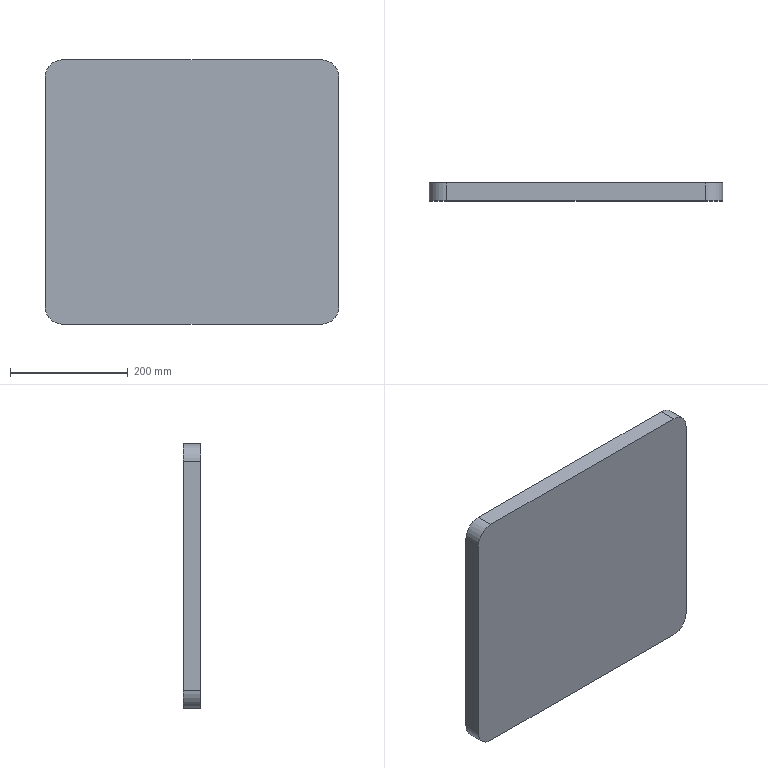Part | SolidWorks | features Extrusion 1, ICE 1 | 1 solid | 19 faces | box 500 x 30 x 450 mm | volume 1262737 mm3 | plane 11 | cylinder 8 | commonest cylinder face diameters 60 x8
STEP:
#1=CARTESIAN_POINT('',(-250.,0.,195.));
#2=VERTEX_POINT('',#1);
#3=CARTESIAN_POINT('',(-220.,0.,225.));
#4=VERTEX_POINT('',#3);
#5=CARTESIAN_POINT('',(-220.,0.,195.));
#6=DIRECTION('',(0.,1.,0.));
#7=DIRECTION('',(0.,0.,-1.));
#8=AXIS2_PLACEMENT_3D('',#5,#6,#7);
#9=CIRCLE('',#8,30.);
#10=EDGE_CURVE('',#2,#4,#9,.T.);
#11=ORIENTED_EDGE('',*,*,#10,.T.);
#12=CARTESIAN_POINT('',(-220.,30.,225.));
#13=VERTEX_POINT('',#12);
#14=CARTESIAN_POINT('',(-220.,30.,225.));
#15=DIRECTION('',(0.,-1.,0.));
#16=VECTOR('',#15,1000.);
#17=LINE('',#14,#16);
#18=EDGE_CURVE('',#13,#4,#17,.T.);
#19=ORIENTED_EDGE('',*,*,#18,.F.);
#20=CARTESIAN_POINT('',(-250.,30.,195.));
#21=VERTEX_POINT('',#20);
#22=CARTESIAN_POINT('',(-220.,30.,195.));
#23=DIRECTION('',(0.,1.,0.));
#24=DIRECTION('',(0.,0.,-1.));
#25=AXIS2_PLACEMENT_3D('',#22,#23,#24);
#26=CIRCLE('',#25,30.);
#27=EDGE_CURVE('',#21,#13,#26,.T.);
#28=ORIENTED_EDGE('',*,*,#27,.F.);
#29=CARTESIAN_POINT('',(-250.,30.,195.));
#30=DIRECTION('',(0.,-1.,0.));
#31=VECTOR('',#30,1000.);
#32=LINE('',#29,#31);
#33=EDGE_CURVE('',#21,#2,#32,.T.);
#34=ORIENTED_EDGE('',*,*,#33,.T.);
#35=EDGE_LOOP('',(#11,#19,#28,#34));
#36=FACE_OUTER_BOUND('',#35,.T.);
#37=CARTESIAN_POINT('',(-220.,30.,195.));
#38=DIRECTION('',(0.,-1.,0.));
#39=DIRECTION('',(0.,0.,-1.));
#40=AXIS2_PLACEMENT_3D('',#37,#38,#39);
#41=CYLINDRICAL_SURFACE('',#40,30.);
#42=ADVANCED_FACE('',(#36),#41,.T.);
#43=CARTESIAN_POINT('',(220.,0.,225.));
#44=VERTEX_POINT('',#43);
#45=CARTESIAN_POINT('',(-220.,0.,225.));
#46=DIRECTION('',(1.,0.,0.));
#47=VECTOR('',#46,1000.);
#48=LINE('',#45,#47);
#49=EDGE_CURVE('',#4,#44,#48,.T.);
#50=ORIENTED_EDGE('',*,*,#49,.T.);
#51=CARTESIAN_POINT('',(220.,30.,225.));
#52=VERTEX_POINT('',#51);
#53=CARTESIAN_POINT('',(220.,30.,225.));
#54=DIRECTION('',(0.,-1.,0.));
#55=VECTOR('',#54,1000.);
#56=LINE('',#53,#55);
#57=EDGE_CURVE('',#52,#44,#56,.T.);
#58=ORIENTED_EDGE('',*,*,#57,.F.);
#59=CARTESIAN_POINT('',(-220.,30.,225.));
#60=DIRECTION('',(1.,0.,0.));
#61=VECTOR('',#60,1000.);
#62=LINE('',#59,#61);
#63=EDGE_CURVE('',#13,#52,#62,.T.);
#64=ORIENTED_EDGE('',*,*,#63,.F.);
#65=ORIENTED_EDGE('',*,*,#18,.T.);
#66=EDGE_LOOP('',(#50,#58,#64,#65));
#67=FACE_OUTER_BOUND('',#66,.T.);
#68=CARTESIAN_POINT('',(-220.,30.,225.));
#69=DIRECTION('',(0.,0.,-1.));
#70=DIRECTION('',(-1.,0.,0.));
#71=AXIS2_PLACEMENT_3D('',#68,#69,#70);
#72=PLANE('',#71);
#73=ADVANCED_FACE('',(#67),#72,.F.);
#74=CARTESIAN_POINT('',(250.,0.,195.));
#75=VERTEX_POINT('',#74);
#76=CARTESIAN_POINT('',(220.,0.,195.));
#77=DIRECTION('',(0.,1.,0.));
#78=DIRECTION('',(0.,0.,-1.));
#79=AXIS2_PLACEMENT_3D('',#76,#77,#78);
#80=CIRCLE('',#79,30.);
#81=EDGE_CURVE('',#44,#75,#80,.T.);
#82=ORIENTED_EDGE('',*,*,#81,.T.);
#83=CARTESIAN_POINT('',(250.,30.,195.));
#84=VERTEX_POINT('',#83);
#85=CARTESIAN_POINT('',(250.,30.,195.));
#86=DIRECTION('',(0.,-1.,0.));
#87=VECTOR('',#86,1000.);
#88=LINE('',#85,#87);
#89=EDGE_CURVE('',#84,#75,#88,.T.);
#90=ORIENTED_EDGE('',*,*,#89,.F.);
#91=CARTESIAN_POINT('',(220.,30.,195.));
#92=DIRECTION('',(0.,1.,0.));
#93=DIRECTION('',(0.,0.,-1.));
#94=AXIS2_PLACEMENT_3D('',#91,#92,#93);
#95=CIRCLE('',#94,30.);
#96=EDGE_CURVE('',#52,#84,#95,.T.);
#97=ORIENTED_EDGE('',*,*,#96,.F.);
#98=ORIENTED_EDGE('',*,*,#57,.T.);
#99=EDGE_LOOP('',(#82,#90,#97,#98));
#100=FACE_OUTER_BOUND('',#99,.T.);
#101=CARTESIAN_POINT('',(220.,30.,195.));
#102=DIRECTION('',(0.,-1.,0.));
#103=DIRECTION('',(0.,0.,-1.));
#104=AXIS2_PLACEMENT_3D('',#101,#102,#103);
#105=CYLINDRICAL_SURFACE('',#104,30.);
#106=ADVANCED_FACE('',(#100),#105,.T.);
#107=CARTESIAN_POINT('',(250.,0.,-195.));
#108=VERTEX_POINT('',#107);
#109=CARTESIAN_POINT('',(250.,0.,-195.));
#110=DIRECTION('',(0.,0.,-1.));
#111=VECTOR('',#110,1000.);
#112=LINE('',#109,#111);
#113=EDGE_CURVE('',#75,#108,#112,.T.);
#114=ORIENTED_EDGE('',*,*,#113,.T.);
#115=CARTESIAN_POINT('',(250.,30.,-195.));
#116=VERTEX_POINT('',#115);
#117=CARTESIAN_POINT('',(250.,30.,-195.));
#118=DIRECTION('',(0.,-1.,0.));
#119=VECTOR('',#118,1000.);
#120=LINE('',#117,#119);
#121=EDGE_CURVE('',#116,#108,#120,.T.);
#122=ORIENTED_EDGE('',*,*,#121,.F.);
#123=CARTESIAN_POINT('',(250.,30.,-195.));
#124=DIRECTION('',(0.,0.,-1.));
#125=VECTOR('',#124,1000.);
#126=LINE('',#123,#125);
#127=EDGE_CURVE('',#84,#116,#126,.T.);
#128=ORIENTED_EDGE('',*,*,#127,.F.);
#129=ORIENTED_EDGE('',*,*,#89,.T.);
#130=EDGE_LOOP('',(#114,#122,#128,#129));
#131=FACE_OUTER_BOUND('',#130,.T.);
#132=CARTESIAN_POINT('',(250.,30.,-195.));
#133=DIRECTION('',(-1.,0.,0.));
#134=DIRECTION('',(0.,0.,1.));
#135=AXIS2_PLACEMENT_3D('',#132,#133,#134);
#136=PLANE('',#135);
#137=ADVANCED_FACE('',(#131),#136,.F.);
#138=CARTESIAN_POINT('',(220.,0.,-225.));
#139=VERTEX_POINT('',#138);
#140=CARTESIAN_POINT('',(220.,0.,-195.));
#141=DIRECTION('',(0.,1.,0.));
#142=DIRECTION('',(0.,0.,1.));
#143=AXIS2_PLACEMENT_3D('',#140,#141,#142);
#144=CIRCLE('',#143,30.);
#145=EDGE_CURVE('',#108,#139,#144,.T.);
#146=ORIENTED_EDGE('',*,*,#145,.T.);
#147=CARTESIAN_POINT('',(220.,30.,-225.));
#148=VERTEX_POINT('',#147);
#149=CARTESIAN_POINT('',(220.,30.,-225.));
#150=DIRECTION('',(0.,-1.,0.));
#151=VECTOR('',#150,1000.);
#152=LINE('',#149,#151);
#153=EDGE_CURVE('',#148,#139,#152,.T.);
#154=ORIENTED_EDGE('',*,*,#153,.F.);
#155=CARTESIAN_POINT('',(220.,30.,-195.));
#156=DIRECTION('',(0.,1.,0.));
#157=DIRECTION('',(0.,0.,1.));
#158=AXIS2_PLACEMENT_3D('',#155,#156,#157);
#159=CIRCLE('',#158,30.);
#160=EDGE_CURVE('',#116,#148,#159,.T.);
#161=ORIENTED_EDGE('',*,*,#160,.F.);
#162=ORIENTED_EDGE('',*,*,#121,.T.);
#163=EDGE_LOOP('',(#146,#154,#161,#162));
#164=FACE_OUTER_BOUND('',#163,.T.);
#165=CARTESIAN_POINT('',(220.,30.,-195.));
#166=DIRECTION('',(0.,-1.,0.));
#167=DIRECTION('',(0.,0.,-1.));
#168=AXIS2_PLACEMENT_3D('',#165,#166,#167);
#169=CYLINDRICAL_SURFACE('',#168,30.);
#170=ADVANCED_FACE('',(#164),#169,.T.);
#171=CARTESIAN_POINT('',(-220.,0.,-225.));
#172=VERTEX_POINT('',#171);
#173=CARTESIAN_POINT('',(-220.,0.,-225.));
#174=DIRECTION('',(-1.,0.,0.));
#175=VECTOR('',#174,1000.);
#176=LINE('',#173,#175);
#177=EDGE_CURVE('',#139,#172,#176,.T.);
#178=ORIENTED_EDGE('',*,*,#177,.T.);
#179=CARTESIAN_POINT('',(-220.,30.,-225.));
#180=VERTEX_POINT('',#179);
#181=CARTESIAN_POINT('',(-220.,30.,-225.));
#182=DIRECTION('',(0.,-1.,0.));
#183=VECTOR('',#182,1000.);
#184=LINE('',#181,#183);
#185=EDGE_CURVE('',#180,#172,#184,.T.);
#186=ORIENTED_EDGE('',*,*,#185,.F.);
#187=CARTESIAN_POINT('',(-220.,30.,-225.));
#188=DIRECTION('',(-1.,0.,0.));
#189=VECTOR('',#188,1000.);
#190=LINE('',#187,#189);
#191=EDGE_CURVE('',#148,#180,#190,.T.);
#192=ORIENTED_EDGE('',*,*,#191,.F.);
#193=ORIENTED_EDGE('',*,*,#153,.T.);
#194=EDGE_LOOP('',(#178,#186,#192,#193));
#195=FACE_OUTER_BOUND('',#194,.T.);
#196=CARTESIAN_POINT('',(-220.,30.,-225.));
#197=DIRECTION('',(0.,0.,1.));
#198=DIRECTION('',(1.,0.,0.));
#199=AXIS2_PLACEMENT_3D('',#196,#197,#198);
#200=PLANE('',#199);
#201=ADVANCED_FACE('',(#195),#200,.F.);
#202=CARTESIAN_POINT('',(-250.,0.,-195.));
#203=VERTEX_POINT('',#202);
#204=CARTESIAN_POINT('',(-220.,0.,-195.));
#205=DIRECTION('',(0.,1.,0.));
#206=DIRECTION('',(0.,0.,1.));
#207=AXIS2_PLACEMENT_3D('',#204,#205,#206);
#208=CIRCLE('',#207,30.);
#209=EDGE_CURVE('',#172,#203,#208,.T.);
#210=ORIENTED_EDGE('',*,*,#209,.T.);
#211=CARTESIAN_POINT('',(-250.,30.,-195.));
#212=VERTEX_POINT('',#211);
#213=CARTESIAN_POINT('',(-250.,30.,-195.));
#214=DIRECTION('',(0.,-1.,0.));
#215=VECTOR('',#214,1000.);
#216=LINE('',#213,#215);
#217=EDGE_CURVE('',#212,#203,#216,.T.);
#218=ORIENTED_EDGE('',*,*,#217,.F.);
#219=CARTESIAN_POINT('',(-220.,30.,-195.));
#220=DIRECTION('',(0.,1.,0.));
#221=DIRECTION('',(0.,0.,1.));
#222=AXIS2_PLACEMENT_3D('',#219,#220,#221);
#223=CIRCLE('',#222,30.);
#224=EDGE_CURVE('',#180,#212,#223,.T.);
#225=ORIENTED_EDGE('',*,*,#224,.F.);
#226=ORIENTED_EDGE('',*,*,#185,.T.);
#227=EDGE_LOOP('',(#210,#218,#225,#226));
#228=FACE_OUTER_BOUND('',#227,.T.);
#229=CARTESIAN_POINT('',(-220.,30.,-195.));
#230=DIRECTION('',(0.,-1.,0.));
#231=DIRECTION('',(0.,0.,-1.));
#232=AXIS2_PLACEMENT_3D('',#229,#230,#231);
#233=CYLINDRICAL_SURFACE('',#232,30.);
#234=ADVANCED_FACE('',(#228),#233,.T.);
#235=CARTESIAN_POINT('',(-250.,0.,-195.));
#236=DIRECTION('',(0.,0.,1.));
#237=VECTOR('',#236,1000.);
#238=LINE('',#235,#237);
#239=EDGE_CURVE('',#203,#2,#238,.T.);
#240=ORIENTED_EDGE('',*,*,#239,.T.);
#241=ORIENTED_EDGE('',*,*,#33,.F.);
#242=CARTESIAN_POINT('',(-250.,30.,-195.));
#243=DIRECTION('',(0.,0.,1.));
#244=VECTOR('',#243,1000.);
#245=LINE('',#242,#244);
#246=EDGE_CURVE('',#212,#21,#245,.T.);
#247=ORIENTED_EDGE('',*,*,#246,.F.);
#248=ORIENTED_EDGE('',*,*,#217,.T.);
#249=EDGE_LOOP('',(#240,#241,#247,#248));
#250=FACE_OUTER_BOUND('',#249,.T.);
#251=CARTESIAN_POINT('',(-250.,30.,-195.));
#252=DIRECTION('',(1.,0.,0.));
#253=DIRECTION('',(0.,0.,-1.));
#254=AXIS2_PLACEMENT_3D('',#251,#252,#253);
#255=PLANE('',#254);
#256=ADVANCED_FACE('',(#250),#255,.F.);
#257=CARTESIAN_POINT('',(247.,30.,192.));
#258=VERTEX_POINT('',#257);
#259=CARTESIAN_POINT('',(247.,30.,-192.));
#260=VERTEX_POINT('',#259);
#261=CARTESIAN_POINT('',(247.,30.,-192.));
#262=DIRECTION('',(0.,0.,-1.));
#263=VECTOR('',#262,1000.);
#264=LINE('',#261,#263);
#265=EDGE_CURVE('',#258,#260,#264,.T.);
#266=ORIENTED_EDGE('',*,*,#265,.F.);
#267=CARTESIAN_POINT('',(217.,30.,222.));
#268=VERTEX_POINT('',#267);
#269=CARTESIAN_POINT('',(217.,30.,192.));
#270=DIRECTION('',(0.,1.,0.));
#271=DIRECTION('',(0.,0.,1.));
#272=AXIS2_PLACEMENT_3D('',#269,#270,#271);
#273=CIRCLE('',#272,30.);
#274=EDGE_CURVE('',#268,#258,#273,.T.);
#275=ORIENTED_EDGE('',*,*,#274,.F.);
#276=CARTESIAN_POINT('',(-217.,30.,222.));
#277=VERTEX_POINT('',#276);
#278=CARTESIAN_POINT('',(-217.,30.,222.));
#279=DIRECTION('',(1.,0.,0.));
#280=VECTOR('',#279,1000.);
#281=LINE('',#278,#280);
#282=EDGE_CURVE('',#277,#268,#281,.T.);
#283=ORIENTED_EDGE('',*,*,#282,.F.);
#284=CARTESIAN_POINT('',(-247.,30.,192.));
#285=VERTEX_POINT('',#284);
#286=CARTESIAN_POINT('',(-217.,30.,192.));
#287=DIRECTION('',(0.,1.,0.));
#288=DIRECTION('',(0.,0.,1.));
#289=AXIS2_PLACEMENT_3D('',#286,#287,#288);
#290=CIRCLE('',#289,30.);
#291=EDGE_CURVE('',#285,#277,#290,.T.);
#292=ORIENTED_EDGE('',*,*,#291,.F.);
#293=CARTESIAN_POINT('',(-247.,30.,-192.));
#294=VERTEX_POINT('',#293);
#295=CARTESIAN_POINT('',(-247.,30.,-192.));
#296=DIRECTION('',(0.,0.,1.));
#297=VECTOR('',#296,1000.);
#298=LINE('',#295,#297);
#299=EDGE_CURVE('',#294,#285,#298,.T.);
#300=ORIENTED_EDGE('',*,*,#299,.F.);
#301=CARTESIAN_POINT('',(-217.,30.,-222.));
#302=VERTEX_POINT('',#301);
#303=CARTESIAN_POINT('',(-217.,30.,-192.));
#304=DIRECTION('',(0.,1.,0.));
#305=DIRECTION('',(0.,0.,-1.));
#306=AXIS2_PLACEMENT_3D('',#303,#304,#305);
#307=CIRCLE('',#306,30.);
#308=EDGE_CURVE('',#302,#294,#307,.T.);
#309=ORIENTED_EDGE('',*,*,#308,.F.);
#310=CARTESIAN_POINT('',(217.,30.,-222.));
#311=VERTEX_POINT('',#310);
#312=CARTESIAN_POINT('',(-217.,30.,-222.));
#313=DIRECTION('',(-1.,0.,0.));
#314=VECTOR('',#313,1000.);
#315=LINE('',#312,#314);
#316=EDGE_CURVE('',#311,#302,#315,.T.);
#317=ORIENTED_EDGE('',*,*,#316,.F.);
#318=CARTESIAN_POINT('',(217.,30.,-192.));
#319=DIRECTION('',(0.,1.,0.));
#320=DIRECTION('',(0.,0.,1.));
#321=AXIS2_PLACEMENT_3D('',#318,#319,#320);
#322=CIRCLE('',#321,30.);
#323=EDGE_CURVE('',#260,#311,#322,.T.);
#324=ORIENTED_EDGE('',*,*,#323,.F.);
#325=EDGE_LOOP('',(#266,#275,#283,#292,#300,#309,#317,#324));
#326=FACE_BOUND('',#325,.T.);
#327=ORIENTED_EDGE('',*,*,#27,.T.);
#328=ORIENTED_EDGE('',*,*,#63,.T.);
#329=ORIENTED_EDGE('',*,*,#96,.T.);
#330=ORIENTED_EDGE('',*,*,#127,.T.);
#331=ORIENTED_EDGE('',*,*,#160,.T.);
#332=ORIENTED_EDGE('',*,*,#191,.T.);
#333=ORIENTED_EDGE('',*,*,#224,.T.);
#334=ORIENTED_EDGE('',*,*,#246,.T.);
#335=EDGE_LOOP('',(#327,#328,#329,#330,#331,#332,#333,#334));
#336=FACE_OUTER_BOUND('',#335,.T.);
#337=CARTESIAN_POINT('',(-220.,30.,195.));
#338=DIRECTION('',(0.,-1.,0.));
#339=DIRECTION('',(0.,0.,-1.));
#340=AXIS2_PLACEMENT_3D('',#337,#338,#339);
#341=PLANE('',#340);
#342=ADVANCED_FACE('',(#326,#336),#341,.F.);
#343=ORIENTED_EDGE('',*,*,#10,.F.);
#344=ORIENTED_EDGE('',*,*,#239,.F.);
#345=ORIENTED_EDGE('',*,*,#209,.F.);
#346=ORIENTED_EDGE('',*,*,#177,.F.);
#347=ORIENTED_EDGE('',*,*,#145,.F.);
#348=ORIENTED_EDGE('',*,*,#113,.F.);
#349=ORIENTED_EDGE('',*,*,#81,.F.);
#350=ORIENTED_EDGE('',*,*,#49,.F.);
#351=EDGE_LOOP('',(#343,#344,#345,#346,#347,#348,#349,#350));
#352=FACE_OUTER_BOUND('',#351,.T.);
#353=CARTESIAN_POINT('',(-220.,0.,195.));
#354=DIRECTION('',(0.,-1.,0.));
#355=DIRECTION('',(0.,0.,-1.));
#356=AXIS2_PLACEMENT_3D('',#353,#354,#355);
#357=PLANE('',#356);
#358=ADVANCED_FACE('',(#352),#357,.T.);
#359=ORIENTED_EDGE('',*,*,#274,.T.);
#360=CARTESIAN_POINT('',(247.,5.,192.));
#361=VERTEX_POINT('',#360);
#362=CARTESIAN_POINT('',(247.,5.,192.));
#363=DIRECTION('',(0.,1.,0.));
#364=VECTOR('',#363,1000.);
#365=LINE('',#362,#364);
#366=EDGE_CURVE('',#361,#258,#365,.T.);
#367=ORIENTED_EDGE('',*,*,#366,.F.);
#368=CARTESIAN_POINT('',(217.,5.,222.));
#369=VERTEX_POINT('',#368);
#370=CARTESIAN_POINT('',(217.,5.,192.));
#371=DIRECTION('',(0.,1.,0.));
#372=DIRECTION('',(0.,0.,1.));
#373=AXIS2_PLACEMENT_3D('',#370,#371,#372);
#374=CIRCLE('',#373,30.);
#375=EDGE_CURVE('',#369,#361,#374,.T.);
#376=ORIENTED_EDGE('',*,*,#375,.F.);
#377=CARTESIAN_POINT('',(217.,5.,222.));
#378=DIRECTION('',(0.,1.,0.));
#379=VECTOR('',#378,1000.);
#380=LINE('',#377,#379);
#381=EDGE_CURVE('',#369,#268,#380,.T.);
#382=ORIENTED_EDGE('',*,*,#381,.T.);
#383=EDGE_LOOP('',(#359,#367,#376,#382));
#384=FACE_OUTER_BOUND('',#383,.T.);
#385=CARTESIAN_POINT('',(217.,5.,192.));
#386=DIRECTION('',(0.,1.,0.));
#387=DIRECTION('',(0.,0.,1.));
#388=AXIS2_PLACEMENT_3D('',#385,#386,#387);
#389=CYLINDRICAL_SURFACE('',#388,30.);
#390=ADVANCED_FACE('',(#384),#389,.F.);
#391=ORIENTED_EDGE('',*,*,#282,.T.);
#392=ORIENTED_EDGE('',*,*,#381,.F.);
#393=CARTESIAN_POINT('',(-217.,5.,222.));
#394=VERTEX_POINT('',#393);
#395=CARTESIAN_POINT('',(-217.,5.,222.));
#396=DIRECTION('',(1.,0.,0.));
#397=VECTOR('',#396,1000.);
#398=LINE('',#395,#397);
#399=EDGE_CURVE('',#394,#369,#398,.T.);
#400=ORIENTED_EDGE('',*,*,#399,.F.);
#401=CARTESIAN_POINT('',(-217.,5.,222.));
#402=DIRECTION('',(0.,1.,0.));
#403=VECTOR('',#402,1000.);
#404=LINE('',#401,#403);
#405=EDGE_CURVE('',#394,#277,#404,.T.);
#406=ORIENTED_EDGE('',*,*,#405,.T.);
#407=EDGE_LOOP('',(#391,#392,#400,#406));
#408=FACE_OUTER_BOUND('',#407,.T.);
#409=CARTESIAN_POINT('',(-217.,5.,222.));
#410=DIRECTION('',(0.,0.,1.));
#411=DIRECTION('',(1.,0.,0.));
#412=AXIS2_PLACEMENT_3D('',#409,#410,#411);
#413=PLANE('',#412);
#414=ADVANCED_FACE('',(#408),#413,.F.);
#415=ORIENTED_EDGE('',*,*,#291,.T.);
#416=ORIENTED_EDGE('',*,*,#405,.F.);
#417=CARTESIAN_POINT('',(-247.,5.,192.));
#418=VERTEX_POINT('',#417);
#419=CARTESIAN_POINT('',(-217.,5.,192.));
#420=DIRECTION('',(0.,1.,0.));
#421=DIRECTION('',(0.,0.,1.));
#422=AXIS2_PLACEMENT_3D('',#419,#420,#421);
#423=CIRCLE('',#422,30.);
#424=EDGE_CURVE('',#418,#394,#423,.T.);
#425=ORIENTED_EDGE('',*,*,#424,.F.);
#426=CARTESIAN_POINT('',(-247.,5.,192.));
#427=DIRECTION('',(0.,1.,0.));
#428=VECTOR('',#427,1000.);
#429=LINE('',#426,#428);
#430=EDGE_CURVE('',#418,#285,#429,.T.);
#431=ORIENTED_EDGE('',*,*,#430,.T.);
#432=EDGE_LOOP('',(#415,#416,#425,#431));
#433=FACE_OUTER_BOUND('',#432,.T.);
#434=CARTESIAN_POINT('',(-217.,5.,192.));
#435=DIRECTION('',(0.,1.,0.));
#436=DIRECTION('',(0.,0.,1.));
#437=AXIS2_PLACEMENT_3D('',#434,#435,#436);
#438=CYLINDRICAL_SURFACE('',#437,30.);
#439=ADVANCED_FACE('',(#433),#438,.F.);
#440=ORIENTED_EDGE('',*,*,#299,.T.);
#441=ORIENTED_EDGE('',*,*,#430,.F.);
#442=CARTESIAN_POINT('',(-247.,5.,-192.));
#443=VERTEX_POINT('',#442);
#444=CARTESIAN_POINT('',(-247.,5.,-192.));
#445=DIRECTION('',(0.,0.,1.));
#446=VECTOR('',#445,1000.);
#447=LINE('',#444,#446);
#448=EDGE_CURVE('',#443,#418,#447,.T.);
#449=ORIENTED_EDGE('',*,*,#448,.F.);
#450=CARTESIAN_POINT('',(-247.,5.,-192.));
#451=DIRECTION('',(0.,1.,0.));
#452=VECTOR('',#451,1000.);
#453=LINE('',#450,#452);
#454=EDGE_CURVE('',#443,#294,#453,.T.);
#455=ORIENTED_EDGE('',*,*,#454,.T.);
#456=EDGE_LOOP('',(#440,#441,#449,#455));
#457=FACE_OUTER_BOUND('',#456,.T.);
#458=CARTESIAN_POINT('',(-247.,5.,-192.));
#459=DIRECTION('',(-1.,0.,0.));
#460=DIRECTION('',(0.,0.,1.));
#461=AXIS2_PLACEMENT_3D('',#458,#459,#460);
#462=PLANE('',#461);
#463=ADVANCED_FACE('',(#457),#462,.F.);
#464=ORIENTED_EDGE('',*,*,#308,.T.);
#465=ORIENTED_EDGE('',*,*,#454,.F.);
#466=CARTESIAN_POINT('',(-217.,5.,-222.));
#467=VERTEX_POINT('',#466);
#468=CARTESIAN_POINT('',(-217.,5.,-192.));
#469=DIRECTION('',(0.,1.,0.));
#470=DIRECTION('',(0.,0.,-1.));
#471=AXIS2_PLACEMENT_3D('',#468,#469,#470);
#472=CIRCLE('',#471,30.);
#473=EDGE_CURVE('',#467,#443,#472,.T.);
#474=ORIENTED_EDGE('',*,*,#473,.F.);
#475=CARTESIAN_POINT('',(-217.,5.,-222.));
#476=DIRECTION('',(0.,1.,0.));
#477=VECTOR('',#476,1000.);
#478=LINE('',#475,#477);
#479=EDGE_CURVE('',#467,#302,#478,.T.);
#480=ORIENTED_EDGE('',*,*,#479,.T.);
#481=EDGE_LOOP('',(#464,#465,#474,#480));
#482=FACE_OUTER_BOUND('',#481,.T.);
#483=CARTESIAN_POINT('',(-217.,5.,-192.));
#484=DIRECTION('',(0.,1.,0.));
#485=DIRECTION('',(0.,0.,1.));
#486=AXIS2_PLACEMENT_3D('',#483,#484,#485);
#487=CYLINDRICAL_SURFACE('',#486,30.);
#488=ADVANCED_FACE('',(#482),#487,.F.);
#489=ORIENTED_EDGE('',*,*,#316,.T.);
#490=ORIENTED_EDGE('',*,*,#479,.F.);
#491=CARTESIAN_POINT('',(217.,5.,-222.));
#492=VERTEX_POINT('',#491);
#493=CARTESIAN_POINT('',(-217.,5.,-222.));
#494=DIRECTION('',(-1.,0.,0.));
#495=VECTOR('',#494,1000.);
#496=LINE('',#493,#495);
#497=EDGE_CURVE('',#492,#467,#496,.T.);
#498=ORIENTED_EDGE('',*,*,#497,.F.);
#499=CARTESIAN_POINT('',(217.,5.,-222.));
#500=DIRECTION('',(0.,1.,0.));
#501=VECTOR('',#500,1000.);
#502=LINE('',#499,#501);
#503=EDGE_CURVE('',#492,#311,#502,.T.);
#504=ORIENTED_EDGE('',*,*,#503,.T.);
#505=EDGE_LOOP('',(#489,#490,#498,#504));
#506=FACE_OUTER_BOUND('',#505,.T.);
#507=CARTESIAN_POINT('',(-217.,5.,-222.));
#508=DIRECTION('',(0.,0.,-1.));
#509=DIRECTION('',(-1.,0.,0.));
#510=AXIS2_PLACEMENT_3D('',#507,#508,#509);
#511=PLANE('',#510);
#512=ADVANCED_FACE('',(#506),#511,.F.);
#513=ORIENTED_EDGE('',*,*,#323,.T.);
#514=ORIENTED_EDGE('',*,*,#503,.F.);
#515=CARTESIAN_POINT('',(247.,5.,-192.));
#516=VERTEX_POINT('',#515);
#517=CARTESIAN_POINT('',(217.,5.,-192.));
#518=DIRECTION('',(0.,1.,0.));
#519=DIRECTION('',(0.,0.,1.));
#520=AXIS2_PLACEMENT_3D('',#517,#518,#519);
#521=CIRCLE('',#520,30.);
#522=EDGE_CURVE('',#516,#492,#521,.T.);
#523=ORIENTED_EDGE('',*,*,#522,.F.);
#524=CARTESIAN_POINT('',(247.,5.,-192.));
#525=DIRECTION('',(0.,1.,0.));
#526=VECTOR('',#525,1000.);
#527=LINE('',#524,#526);
#528=EDGE_CURVE('',#516,#260,#527,.T.);
#529=ORIENTED_EDGE('',*,*,#528,.T.);
#530=EDGE_LOOP('',(#513,#514,#523,#529));
#531=FACE_OUTER_BOUND('',#530,.T.);
#532=CARTESIAN_POINT('',(217.,5.,-192.));
#533=DIRECTION('',(0.,1.,0.));
#534=DIRECTION('',(0.,0.,1.));
#535=AXIS2_PLACEMENT_3D('',#532,#533,#534);
#536=CYLINDRICAL_SURFACE('',#535,30.);
#537=ADVANCED_FACE('',(#531),#536,.F.);
#538=ORIENTED_EDGE('',*,*,#265,.T.);
#539=ORIENTED_EDGE('',*,*,#528,.F.);
#540=CARTESIAN_POINT('',(247.,5.,-192.));
#541=DIRECTION('',(0.,0.,-1.));
#542=VECTOR('',#541,1000.);
#543=LINE('',#540,#542);
#544=EDGE_CURVE('',#361,#516,#543,.T.);
#545=ORIENTED_EDGE('',*,*,#544,.F.);
#546=ORIENTED_EDGE('',*,*,#366,.T.);
#547=EDGE_LOOP('',(#538,#539,#545,#546));
#548=FACE_OUTER_BOUND('',#547,.T.);
#549=CARTESIAN_POINT('',(247.,5.,-192.));
#550=DIRECTION('',(1.,0.,0.));
#551=DIRECTION('',(0.,0.,-1.));
#552=AXIS2_PLACEMENT_3D('',#549,#550,#551);
#553=PLANE('',#552);
#554=ADVANCED_FACE('',(#548),#553,.F.);
#555=ORIENTED_EDGE('',*,*,#375,.T.);
#556=ORIENTED_EDGE('',*,*,#544,.T.);
#557=ORIENTED_EDGE('',*,*,#522,.T.);
#558=ORIENTED_EDGE('',*,*,#497,.T.);
#559=ORIENTED_EDGE('',*,*,#473,.T.);
#560=ORIENTED_EDGE('',*,*,#448,.T.);
#561=ORIENTED_EDGE('',*,*,#424,.T.);
#562=ORIENTED_EDGE('',*,*,#399,.T.);
#563=EDGE_LOOP('',(#555,#556,#557,#558,#559,#560,#561,#562));
#564=FACE_OUTER_BOUND('',#563,.T.);
#565=CARTESIAN_POINT('',(217.,5.,192.));
#566=DIRECTION('',(0.,1.,0.));
#567=DIRECTION('',(0.,0.,1.));
#568=AXIS2_PLACEMENT_3D('',#565,#566,#567);
#569=PLANE('',#568);
#570=ADVANCED_FACE('',(#564),#569,.T.);
#571=CLOSED_SHELL('',(#42,#73,#106,#137,#170,#201,#234,#256,#342,#358,#390,#414,#439,#463,#488,#512,#537,#554,#570));
#572=MANIFOLD_SOLID_BREP('',#571);
#573=CARTESIAN_POINT('',(0.,0.,0.));
#574=DIRECTION('',(0.,0.,1.));
#575=DIRECTION('',(1.,0.,0.));
#576=AXIS2_PLACEMENT_3D('',#573,#574,#575);
#577=(LENGTH_UNIT()NAMED_UNIT(*)SI_UNIT(.MILLI.,.METRE.));
#578=UNCERTAINTY_MEASURE_WITH_UNIT(LENGTH_MEASURE(0.00001),#577,'','');
#579=(NAMED_UNIT(*)PLANE_ANGLE_UNIT()SI_UNIT($,.RADIAN.));
#580=(NAMED_UNIT(*)SI_UNIT($,.STERADIAN.)SOLID_ANGLE_UNIT());
#581=(GEOMETRIC_REPRESENTATION_CONTEXT(3)GLOBAL_UNCERTAINTY_ASSIGNED_CONTEXT((#578))GLOBAL_UNIT_ASSIGNED_CONTEXT((#577,#579,#580))REPRESENTATION_CONTEXT('',''));
#582=ADVANCED_BREP_SHAPE_REPRESENTATION('',(#572,#576),#581);